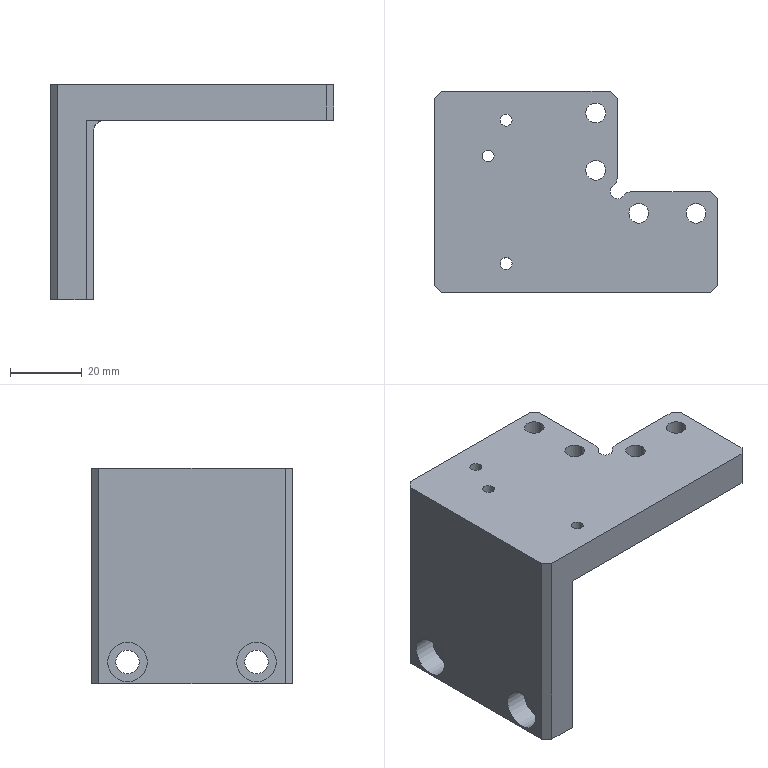CAM job | NX | 3-axis milling, drilling | part box 79 x 56 x 60 mm | stock box 84 x 61 x 65 mm
Tools:
number,name,description,diameter,corner_radius,flute_length,length,flutes
18,D16,平底铣刀-粗,16.0,0.0,50.0,75.0,2
11,D3-J,平底铣刀-精,3.0,0.0,50.0,75.0,2
19,D16-J,平底铣刀-精,16.0,0.0,50.0,75.0,2
1,D80R0.8飞刀,圆鼻刀-粗,80.0,0.8,50.0,75.0,2
1,D80R0.8飞刀-J,圆鼻刀-精,80.0,0.8,50.0,75.0,2
2,D6倒角刀,倒角刀,6.0,0.0,3.0,25.0,2
21,M4X0.7,丝锥,3.3,0.0,35.0,50.0,2
17,ZT5.5,钻头,5.5,0.0,35.0,50.0,2
23,D6-EXTENDED,平底铣刀-粗,6.0,0.0,50.0,75.0,2
13,钻头3.3,Twist Drill 3.3 mm,3.3,0.0,35.0,35.008,2
Operations:
program,operation,operation_type,tool,method,geometry_group,spindle_rpm,surface_speed,feed_per_tooth,feed_cut,feed_plunge,cut_length_mm,path_length_mm,cut_time_min,machine_time_min
B,底壁铣飞面一刀开粗_COPY,VolumeBased25DMillingOperation,D80R0.8飞刀,分层开粗-切深K-步距G,W-B,2800.0,703.696,0.5357,3000.0,100.0,1684.746,3348.967,0.5616,0.728
B,底壁铣飞面一刀精光_COPY,VolumeBased25DMillingOperation,D80R0.8飞刀-J,侧刃精光-切深K-步距G,W-B,4000.0,1005.28,0.125,1000.0,100.0,186.998,222.998,0.187,0.1906
B,型腔铣开粗-中_COPY_1,CavityMilling,D16,分层开粗-切深K-步距G,W-B,6000.0,188.496,0.3333,4000.0,100.0,45041.466,47890.168,11.26,11.696
B,C0.3封闭铣廓倒角6X45L_COPY,PlanarMilling,D6倒角刀,爬面_倒角-切深0-步距G,W-B,7000.0,131.0,0.1071,1500.0,100.0,148.842,184.842,0.0992,0.1028
B,铣沉头_1,CylinderMilling,D6-EXTENDED,METHOD,W-B,3000.0,56.549,0.3333,2000.0,100.0,1886.509,2529.372,0.9433,1.008
B,铣孔_1,CylinderMilling,D6-EXTENDED,METHOD,W-B,3000.0,56.549,0.1,600.0,100.0,70.227,735.89,0.117,0.1836
B,底壁铣精光底面-中_COPY,VolumeBased25DMillingOperation,D16-J,精光步距切深关,W-B,5000.0,251.327,0.1,1000.0,100.0,444.656,570.656,0.4447,0.4573
B,等高精光-中_COPY,ZLevelMilling,D16-J,侧刃精光-切深K-步距G,W-B,5000.0,251.327,0.1,1000.0,100.0,398.04,1061.045,0.398,0.4643
B,底壁铣精光侧面-中-选底面_COPY,VolumeBased25DMillingOperation,D16-J,侧刃精光-切深K-步距G,W-B,5000.0,251.327,0.1,1000.0,100.0,89.353,216.353,0.0894,0.1021
B,等高精光往复爬面_COPY,ZLevelMilling,D16-J,等高爬面-切深K-步距G,W-B,5000.0,251.327,0.4,4000.0,100.0,21199.165,21324.68,5.3,5.312
A,顶面,FaceMilling,D80R0.8飞刀,侧刃精光-切深K-步距G,W-A,4000.0,1005.31,0.125,1000.0,100.0,173.0,209.0,0.173,0.1766
A,型腔铣开粗-中_COPY,CavityMilling,D16,分层开粗-切深K-步距G,W-A,6000.0,301.593,0.3333,4000.0,100.0,34627.452,37578.637,8.657,9.103
A,外形粗_2,VolumeBased25DMillingOperation,D16,METHOD,W-A,6000.0,301.593,0.4167,5000.0,80.0,23991.65,24090.15,4.798,4.808
A,打点-深0.8,Operation,D6倒角刀,NONE,W-A,8000.0,150.796,0.0312,500.0,90.0,12.6,187.018,0.0252,0.0426
A,通孔-M4螺纹底孔,Operation,钻头3.3,NONE,W-A,3000.0,31.102,0.05,300.0,90.0,33.983,148.978,0.1133,0.1248
A,盲锥孔-M4螺纹底孔,Operation,钻头3.3,NONE,W-A,3000.0,31.102,0.02,120.0,90.0,17.0,74.0,0.1417,0.1474
A,通孔-5-6,Operation,ZT5.5,NONE,W-A,3000.0,51.836,0.025,150.0,90.0,56.0,204.062,0.3733,0.3881
A,外形侧面,ZLevelMilling,D3-J,METHOD,W-A,9000.0,84.823,0.1389,2500.0,80.0,803.976,1433.948,0.3249,0.3879
A,仅选体,SurfaceContour,D6倒角刀,METHOD,W-A,8000.0,150.796,0.1875,3000.0,100.0,285.855,321.656,0.0953,0.0989
A,钻倒角_1,Operation,D6倒角刀,METHOD,W-A,8000.0,150.796,0.0312,500.0,0.0,15.6,119.337,0.0312,0.0416
A,铣倒角_1,PlanarMilling,D6倒角刀,METHOD,W-A,8000.0,150.796,0.0312,500.0,100.0,78.753,288.541,0.1575,0.1785
A,通孔-攻牙M4,Operation,M4X0.7,METHOD,W-A,600.0,6.22,0.0006,0.7,90.0,28.0,137.012,40.0,40.011
A,盲锥孔-攻牙M4,Operation,M4X0.7,METHOD,W-A,800.0,8.294,0.0004,0.7,90.0,14.0,68.0,20.0,20.005
A,外形半精_2,VolumeBased25DMillingOperation,D16-J,METHOD,W-A,6000.0,301.593,0.0833,1000.0,100.0,947.88,1309.9,0.9479,0.9841